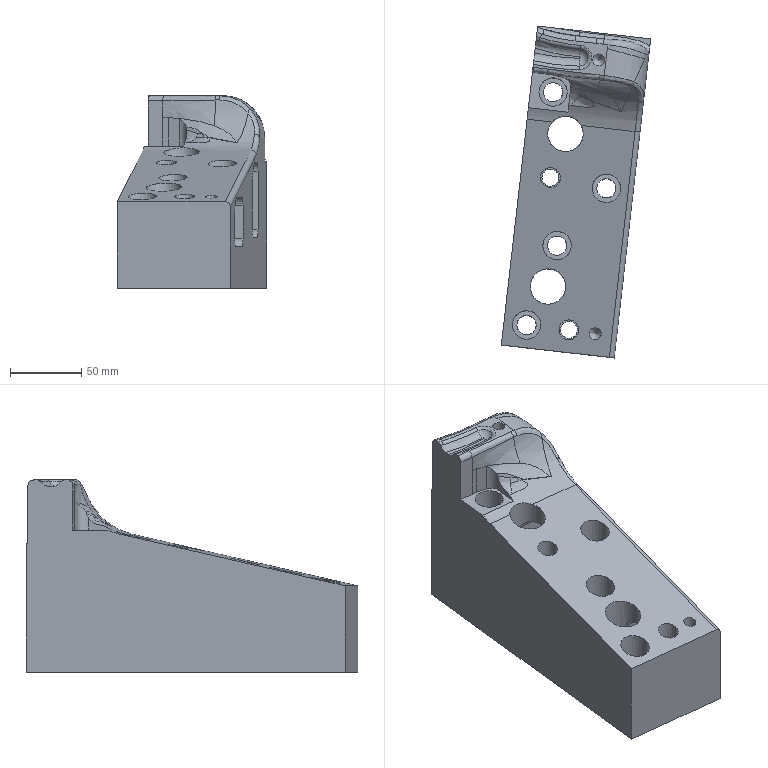Part | NX | features 23 2 | 1 solid | 129 faces | box 106.78 x 233.604 x 135.4 mm | volume 1327898 mm3 | cylinder 50 | plane 44 | spline 25 | torus 8 | cone 2 | commonest cylinder face diameters 12 x10 9.75 x8 7 x5 13.5 x4 20 x4 14 x3